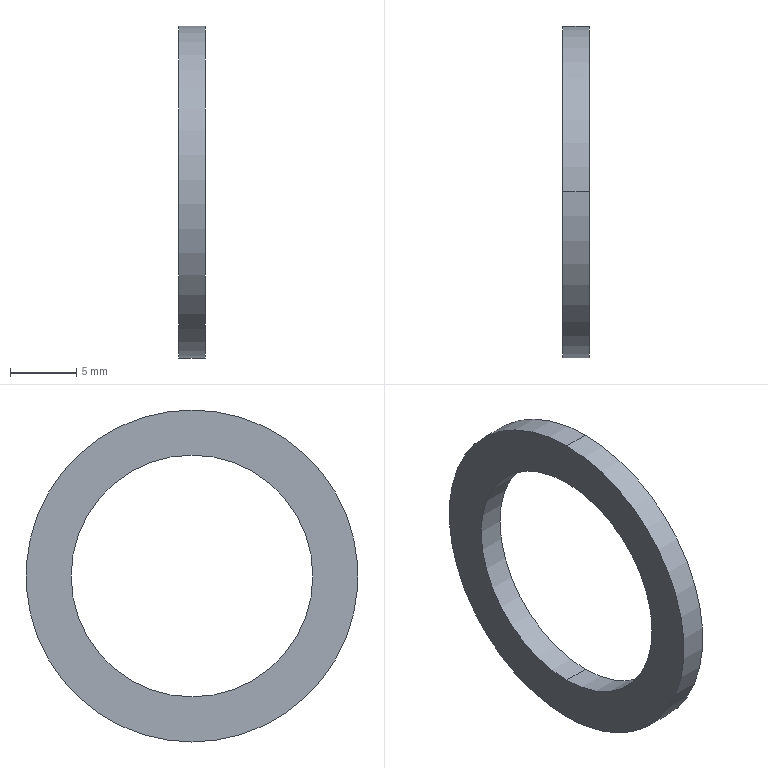Part | STEP file | PN_0010 positioning ring_Default | 1 solid | 6 faces | box 2 x 25 x 25 mm | volume 461.437 mm3 | cylinder 4 | plane 2 | commonest cylinder face diameters 18.2 x2 25 x2
STEP:
#1=CARTESIAN_POINT('',(0.,0.,0.));
#2=DIRECTION('',(0.,0.,1.));
#3=DIRECTION('',(1.,0.,0.));
#4=AXIS2_PLACEMENT_3D('',#1,#2,#3);
#5=CARTESIAN_POINT('',(2.,0.,9.1));
#6=VERTEX_POINT('',#5);
#7=CARTESIAN_POINT('',(0.,0.,9.1));
#8=VERTEX_POINT('',#7);
#9=CARTESIAN_POINT('',(2.,0.,9.1));
#10=DIRECTION('',(-1.,0.,0.));
#11=VECTOR('',#10,1.);
#12=LINE('',#9,#11);
#13=CARTESIAN_POINT('',(2.,0.,0.));
#14=DIRECTION('',(-1.,0.,0.));
#15=DIRECTION('',(0.,0.,1.));
#16=AXIS2_PLACEMENT_3D('',#13,#14,#15);
#17=CYLINDRICAL_SURFACE('',#16,9.1);
#18=CARTESIAN_POINT('',(6.283,0.));
#19=DIRECTION('',(0.,1.));
#20=VECTOR('',#19,1.);
#21=LINE('',#18,#20);
#22=(GEOMETRIC_REPRESENTATION_CONTEXT(2)PARAMETRIC_REPRESENTATION_CONTEXT()REPRESENTATION_CONTEXT('',''));
#23=DEFINITIONAL_REPRESENTATION('',(#21),#22);
#24=PCURVE('',#17,#23);
#25=CARTESIAN_POINT('',(2.,0.,0.));
#26=DIRECTION('',(-1.,0.,0.));
#27=DIRECTION('',(0.,0.,1.));
#28=AXIS2_PLACEMENT_3D('',#25,#26,#27);
#29=CYLINDRICAL_SURFACE('',#28,9.1);
#30=CARTESIAN_POINT('',(0.,0.));
#31=DIRECTION('',(0.,1.));
#32=VECTOR('',#31,1.);
#33=LINE('',#30,#32);
#34=(GEOMETRIC_REPRESENTATION_CONTEXT(2)PARAMETRIC_REPRESENTATION_CONTEXT()REPRESENTATION_CONTEXT('',''));
#35=DEFINITIONAL_REPRESENTATION('',(#33),#34);
#36=PCURVE('',#29,#35);
#37=SURFACE_CURVE('',#12,(#24,#36),.PCURVE_S1.);
#38=EDGE_CURVE('',#6,#8,#37,.T.);
#39=ORIENTED_EDGE('',*,*,#38,.T.);
#40=CARTESIAN_POINT('',(0.,0.,-9.1));
#41=VERTEX_POINT('',#40);
#42=CARTESIAN_POINT('',(0.,0.,0.));
#43=DIRECTION('',(1.,0.,0.));
#44=DIRECTION('',(0.,0.,-1.));
#45=AXIS2_PLACEMENT_3D('',#42,#43,#44);
#46=CIRCLE('',#45,9.1);
#47=CARTESIAN_POINT('',(9.425,2.));
#48=DIRECTION('',(-1.,0.));
#49=VECTOR('',#48,1.);
#50=LINE('',#47,#49);
#51=(GEOMETRIC_REPRESENTATION_CONTEXT(2)PARAMETRIC_REPRESENTATION_CONTEXT()REPRESENTATION_CONTEXT('',''));
#52=DEFINITIONAL_REPRESENTATION('',(#50),#51);
#53=PCURVE('',#17,#52);
#54=CARTESIAN_POINT('',(0.,0.,0.));
#55=DIRECTION('',(1.,0.,0.));
#56=DIRECTION('',(0.,0.,-1.));
#57=AXIS2_PLACEMENT_3D('',#54,#55,#56);
#58=PLANE('',#57);
#59=CARTESIAN_POINT('',(0.,0.));
#60=DIRECTION('',(1.,0.));
#61=AXIS2_PLACEMENT_2D('',#59,#60);
#62=CIRCLE('',#61,9.1);
#63=(GEOMETRIC_REPRESENTATION_CONTEXT(2)PARAMETRIC_REPRESENTATION_CONTEXT()REPRESENTATION_CONTEXT('',''));
#64=DEFINITIONAL_REPRESENTATION('',(#62),#63);
#65=PCURVE('',#58,#64);
#66=SURFACE_CURVE('',#46,(#53,#65),.PCURVE_S1.);
#67=EDGE_CURVE('',#8,#41,#66,.T.);
#68=ORIENTED_EDGE('',*,*,#67,.T.);
#69=CARTESIAN_POINT('',(2.,0.,-9.1));
#70=VERTEX_POINT('',#69);
#71=CARTESIAN_POINT('',(2.,0.,-9.1));
#72=DIRECTION('',(-1.,0.,0.));
#73=VECTOR('',#72,1.);
#74=LINE('',#71,#73);
#75=CARTESIAN_POINT('',(3.142,0.));
#76=DIRECTION('',(0.,1.));
#77=VECTOR('',#76,1.);
#78=LINE('',#75,#77);
#79=(GEOMETRIC_REPRESENTATION_CONTEXT(2)PARAMETRIC_REPRESENTATION_CONTEXT()REPRESENTATION_CONTEXT('',''));
#80=DEFINITIONAL_REPRESENTATION('',(#78),#79);
#81=PCURVE('',#17,#80);
#82=CARTESIAN_POINT('',(3.142,0.));
#83=DIRECTION('',(0.,1.));
#84=VECTOR('',#83,1.);
#85=LINE('',#82,#84);
#86=(GEOMETRIC_REPRESENTATION_CONTEXT(2)PARAMETRIC_REPRESENTATION_CONTEXT()REPRESENTATION_CONTEXT('',''));
#87=DEFINITIONAL_REPRESENTATION('',(#85),#86);
#88=PCURVE('',#29,#87);
#89=SURFACE_CURVE('',#74,(#81,#88),.PCURVE_S1.);
#90=EDGE_CURVE('',#70,#41,#89,.T.);
#91=ORIENTED_EDGE('',*,*,#90,.F.);
#92=CARTESIAN_POINT('',(2.,0.,0.));
#93=DIRECTION('',(1.,0.,0.));
#94=DIRECTION('',(0.,0.,-1.));
#95=AXIS2_PLACEMENT_3D('',#92,#93,#94);
#96=CIRCLE('',#95,9.1);
#97=CARTESIAN_POINT('',(9.425,0.));
#98=DIRECTION('',(-1.,0.));
#99=VECTOR('',#98,1.);
#100=LINE('',#97,#99);
#101=(GEOMETRIC_REPRESENTATION_CONTEXT(2)PARAMETRIC_REPRESENTATION_CONTEXT()REPRESENTATION_CONTEXT('',''));
#102=DEFINITIONAL_REPRESENTATION('',(#100),#101);
#103=PCURVE('',#17,#102);
#104=CARTESIAN_POINT('',(2.,0.,0.));
#105=DIRECTION('',(1.,0.,0.));
#106=DIRECTION('',(0.,0.,-1.));
#107=AXIS2_PLACEMENT_3D('',#104,#105,#106);
#108=PLANE('',#107);
#109=CARTESIAN_POINT('',(0.,0.));
#110=DIRECTION('',(1.,0.));
#111=AXIS2_PLACEMENT_2D('',#109,#110);
#112=CIRCLE('',#111,9.1);
#113=(GEOMETRIC_REPRESENTATION_CONTEXT(2)PARAMETRIC_REPRESENTATION_CONTEXT()REPRESENTATION_CONTEXT('',''));
#114=DEFINITIONAL_REPRESENTATION('',(#112),#113);
#115=PCURVE('',#108,#114);
#116=SURFACE_CURVE('',#96,(#103,#115),.PCURVE_S1.);
#117=EDGE_CURVE('',#6,#70,#116,.T.);
#118=ORIENTED_EDGE('',*,*,#117,.F.);
#119=EDGE_LOOP('',(#39,#68,#91,#118));
#120=FACE_BOUND('',#119,.F.);
#121=ADVANCED_FACE('',(#120),#17,.F.);
#122=CARTESIAN_POINT('',(2.,0.,-12.5));
#123=VERTEX_POINT('',#122);
#124=CARTESIAN_POINT('',(2.,0.,12.5));
#125=VERTEX_POINT('',#124);
#126=CARTESIAN_POINT('',(2.,0.,0.));
#127=DIRECTION('',(1.,0.,0.));
#128=DIRECTION('',(0.,0.,-1.));
#129=AXIS2_PLACEMENT_3D('',#126,#127,#128);
#130=CIRCLE('',#129,12.5);
#131=CARTESIAN_POINT('',(2.,0.,0.));
#132=DIRECTION('',(-1.,0.,0.));
#133=DIRECTION('',(0.,0.,1.));
#134=AXIS2_PLACEMENT_3D('',#131,#132,#133);
#135=CYLINDRICAL_SURFACE('',#134,12.5);
#136=CARTESIAN_POINT('',(3.142,0.));
#137=DIRECTION('',(-1.,0.));
#138=VECTOR('',#137,1.);
#139=LINE('',#136,#138);
#140=(GEOMETRIC_REPRESENTATION_CONTEXT(2)PARAMETRIC_REPRESENTATION_CONTEXT()REPRESENTATION_CONTEXT('',''));
#141=DEFINITIONAL_REPRESENTATION('',(#139),#140);
#142=PCURVE('',#135,#141);
#143=CARTESIAN_POINT('',(0.,0.));
#144=DIRECTION('',(1.,0.));
#145=AXIS2_PLACEMENT_2D('',#143,#144);
#146=CIRCLE('',#145,12.5);
#147=(GEOMETRIC_REPRESENTATION_CONTEXT(2)PARAMETRIC_REPRESENTATION_CONTEXT()REPRESENTATION_CONTEXT('',''));
#148=DEFINITIONAL_REPRESENTATION('',(#146),#147);
#149=PCURVE('',#108,#148);
#150=SURFACE_CURVE('',#130,(#142,#149),.PCURVE_S1.);
#151=EDGE_CURVE('',#123,#125,#150,.T.);
#152=ORIENTED_EDGE('',*,*,#151,.F.);
#153=CARTESIAN_POINT('',(0.,0.,-12.5));
#154=VERTEX_POINT('',#153);
#155=CARTESIAN_POINT('',(2.,0.,-12.5));
#156=DIRECTION('',(-1.,0.,0.));
#157=VECTOR('',#156,1.);
#158=LINE('',#155,#157);
#159=CARTESIAN_POINT('',(3.142,0.));
#160=DIRECTION('',(0.,1.));
#161=VECTOR('',#160,1.);
#162=LINE('',#159,#161);
#163=(GEOMETRIC_REPRESENTATION_CONTEXT(2)PARAMETRIC_REPRESENTATION_CONTEXT()REPRESENTATION_CONTEXT('',''));
#164=DEFINITIONAL_REPRESENTATION('',(#162),#163);
#165=PCURVE('',#135,#164);
#166=CARTESIAN_POINT('',(2.,0.,0.));
#167=DIRECTION('',(-1.,0.,0.));
#168=DIRECTION('',(0.,0.,1.));
#169=AXIS2_PLACEMENT_3D('',#166,#167,#168);
#170=CYLINDRICAL_SURFACE('',#169,12.5);
#171=CARTESIAN_POINT('',(3.142,0.));
#172=DIRECTION('',(0.,1.));
#173=VECTOR('',#172,1.);
#174=LINE('',#171,#173);
#175=(GEOMETRIC_REPRESENTATION_CONTEXT(2)PARAMETRIC_REPRESENTATION_CONTEXT()REPRESENTATION_CONTEXT('',''));
#176=DEFINITIONAL_REPRESENTATION('',(#174),#175);
#177=PCURVE('',#170,#176);
#178=SURFACE_CURVE('',#158,(#165,#177),.PCURVE_S1.);
#179=EDGE_CURVE('',#123,#154,#178,.T.);
#180=ORIENTED_EDGE('',*,*,#179,.T.);
#181=CARTESIAN_POINT('',(0.,0.,12.5));
#182=VERTEX_POINT('',#181);
#183=CARTESIAN_POINT('',(0.,0.,0.));
#184=DIRECTION('',(1.,0.,0.));
#185=DIRECTION('',(0.,0.,-1.));
#186=AXIS2_PLACEMENT_3D('',#183,#184,#185);
#187=CIRCLE('',#186,12.5);
#188=CARTESIAN_POINT('',(3.142,2.));
#189=DIRECTION('',(-1.,0.));
#190=VECTOR('',#189,1.);
#191=LINE('',#188,#190);
#192=(GEOMETRIC_REPRESENTATION_CONTEXT(2)PARAMETRIC_REPRESENTATION_CONTEXT()REPRESENTATION_CONTEXT('',''));
#193=DEFINITIONAL_REPRESENTATION('',(#191),#192);
#194=PCURVE('',#135,#193);
#195=CARTESIAN_POINT('',(0.,0.));
#196=DIRECTION('',(1.,0.));
#197=AXIS2_PLACEMENT_2D('',#195,#196);
#198=CIRCLE('',#197,12.5);
#199=(GEOMETRIC_REPRESENTATION_CONTEXT(2)PARAMETRIC_REPRESENTATION_CONTEXT()REPRESENTATION_CONTEXT('',''));
#200=DEFINITIONAL_REPRESENTATION('',(#198),#199);
#201=PCURVE('',#58,#200);
#202=SURFACE_CURVE('',#187,(#194,#201),.PCURVE_S1.);
#203=EDGE_CURVE('',#154,#182,#202,.T.);
#204=ORIENTED_EDGE('',*,*,#203,.T.);
#205=CARTESIAN_POINT('',(2.,0.,12.5));
#206=DIRECTION('',(-1.,0.,0.));
#207=VECTOR('',#206,1.);
#208=LINE('',#205,#207);
#209=CARTESIAN_POINT('',(0.,0.));
#210=DIRECTION('',(0.,1.));
#211=VECTOR('',#210,1.);
#212=LINE('',#209,#211);
#213=(GEOMETRIC_REPRESENTATION_CONTEXT(2)PARAMETRIC_REPRESENTATION_CONTEXT()REPRESENTATION_CONTEXT('',''));
#214=DEFINITIONAL_REPRESENTATION('',(#212),#213);
#215=PCURVE('',#135,#214);
#216=CARTESIAN_POINT('',(6.283,0.));
#217=DIRECTION('',(0.,1.));
#218=VECTOR('',#217,1.);
#219=LINE('',#216,#218);
#220=(GEOMETRIC_REPRESENTATION_CONTEXT(2)PARAMETRIC_REPRESENTATION_CONTEXT()REPRESENTATION_CONTEXT('',''));
#221=DEFINITIONAL_REPRESENTATION('',(#219),#220);
#222=PCURVE('',#170,#221);
#223=SURFACE_CURVE('',#208,(#215,#222),.PCURVE_S1.);
#224=EDGE_CURVE('',#125,#182,#223,.T.);
#225=ORIENTED_EDGE('',*,*,#224,.F.);
#226=EDGE_LOOP('',(#152,#180,#204,#225));
#227=FACE_BOUND('',#226,.T.);
#228=ADVANCED_FACE('',(#227),#135,.T.);
#229=CARTESIAN_POINT('',(2.,0.,0.));
#230=DIRECTION('',(1.,0.,0.));
#231=DIRECTION('',(0.,0.,-1.));
#232=AXIS2_PLACEMENT_3D('',#229,#230,#231);
#233=CIRCLE('',#232,12.5);
#234=CARTESIAN_POINT('',(0.,0.));
#235=DIRECTION('',(1.,0.));
#236=AXIS2_PLACEMENT_2D('',#234,#235);
#237=CIRCLE('',#236,12.5);
#238=(GEOMETRIC_REPRESENTATION_CONTEXT(2)PARAMETRIC_REPRESENTATION_CONTEXT()REPRESENTATION_CONTEXT('',''));
#239=DEFINITIONAL_REPRESENTATION('',(#237),#238);
#240=PCURVE('',#108,#239);
#241=CARTESIAN_POINT('',(9.425,0.));
#242=DIRECTION('',(-1.,0.));
#243=VECTOR('',#242,1.);
#244=LINE('',#241,#243);
#245=(GEOMETRIC_REPRESENTATION_CONTEXT(2)PARAMETRIC_REPRESENTATION_CONTEXT()REPRESENTATION_CONTEXT('',''));
#246=DEFINITIONAL_REPRESENTATION('',(#244),#245);
#247=PCURVE('',#170,#246);
#248=SURFACE_CURVE('',#233,(#240,#247),.PCURVE_S1.);
#249=EDGE_CURVE('',#125,#123,#248,.T.);
#250=ORIENTED_EDGE('',*,*,#249,.T.);
#251=ORIENTED_EDGE('',*,*,#151,.T.);
#252=EDGE_LOOP('',(#250,#251));
#253=FACE_BOUND('',#252,.T.);
#254=ORIENTED_EDGE('',*,*,#117,.F.);
#255=CARTESIAN_POINT('',(2.,0.,0.));
#256=DIRECTION('',(1.,0.,0.));
#257=DIRECTION('',(0.,0.,-1.));
#258=AXIS2_PLACEMENT_3D('',#255,#256,#257);
#259=CIRCLE('',#258,9.1);
#260=CARTESIAN_POINT('',(0.,0.));
#261=DIRECTION('',(1.,0.));
#262=AXIS2_PLACEMENT_2D('',#260,#261);
#263=CIRCLE('',#262,9.1);
#264=(GEOMETRIC_REPRESENTATION_CONTEXT(2)PARAMETRIC_REPRESENTATION_CONTEXT()REPRESENTATION_CONTEXT('',''));
#265=DEFINITIONAL_REPRESENTATION('',(#263),#264);
#266=PCURVE('',#108,#265);
#267=CARTESIAN_POINT('',(3.142,0.));
#268=DIRECTION('',(-1.,0.));
#269=VECTOR('',#268,1.);
#270=LINE('',#267,#269);
#271=(GEOMETRIC_REPRESENTATION_CONTEXT(2)PARAMETRIC_REPRESENTATION_CONTEXT()REPRESENTATION_CONTEXT('',''));
#272=DEFINITIONAL_REPRESENTATION('',(#270),#271);
#273=PCURVE('',#29,#272);
#274=SURFACE_CURVE('',#259,(#266,#273),.PCURVE_S1.);
#275=EDGE_CURVE('',#70,#6,#274,.T.);
#276=ORIENTED_EDGE('',*,*,#275,.F.);
#277=EDGE_LOOP('',(#254,#276));
#278=FACE_BOUND('',#277,.T.);
#279=ADVANCED_FACE('',(#253,#278),#108,.T.);
#280=CARTESIAN_POINT('',(0.,0.,0.));
#281=DIRECTION('',(1.,0.,0.));
#282=DIRECTION('',(0.,0.,-1.));
#283=AXIS2_PLACEMENT_3D('',#280,#281,#282);
#284=CIRCLE('',#283,12.5);
#285=CARTESIAN_POINT('',(0.,0.));
#286=DIRECTION('',(1.,0.));
#287=AXIS2_PLACEMENT_2D('',#285,#286);
#288=CIRCLE('',#287,12.5);
#289=(GEOMETRIC_REPRESENTATION_CONTEXT(2)PARAMETRIC_REPRESENTATION_CONTEXT()REPRESENTATION_CONTEXT('',''));
#290=DEFINITIONAL_REPRESENTATION('',(#288),#289);
#291=PCURVE('',#58,#290);
#292=CARTESIAN_POINT('',(9.425,2.));
#293=DIRECTION('',(-1.,0.));
#294=VECTOR('',#293,1.);
#295=LINE('',#292,#294);
#296=(GEOMETRIC_REPRESENTATION_CONTEXT(2)PARAMETRIC_REPRESENTATION_CONTEXT()REPRESENTATION_CONTEXT('',''));
#297=DEFINITIONAL_REPRESENTATION('',(#295),#296);
#298=PCURVE('',#170,#297);
#299=SURFACE_CURVE('',#284,(#291,#298),.PCURVE_S1.);
#300=EDGE_CURVE('',#182,#154,#299,.T.);
#301=ORIENTED_EDGE('',*,*,#300,.F.);
#302=ORIENTED_EDGE('',*,*,#203,.F.);
#303=EDGE_LOOP('',(#301,#302));
#304=FACE_BOUND('',#303,.T.);
#305=ORIENTED_EDGE('',*,*,#67,.T.);
#306=CARTESIAN_POINT('',(0.,0.,0.));
#307=DIRECTION('',(1.,0.,0.));
#308=DIRECTION('',(0.,0.,-1.));
#309=AXIS2_PLACEMENT_3D('',#306,#307,#308);
#310=CIRCLE('',#309,9.1);
#311=CARTESIAN_POINT('',(0.,0.));
#312=DIRECTION('',(1.,0.));
#313=AXIS2_PLACEMENT_2D('',#311,#312);
#314=CIRCLE('',#313,9.1);
#315=(GEOMETRIC_REPRESENTATION_CONTEXT(2)PARAMETRIC_REPRESENTATION_CONTEXT()REPRESENTATION_CONTEXT('',''));
#316=DEFINITIONAL_REPRESENTATION('',(#314),#315);
#317=PCURVE('',#58,#316);
#318=CARTESIAN_POINT('',(3.142,2.));
#319=DIRECTION('',(-1.,0.));
#320=VECTOR('',#319,1.);
#321=LINE('',#318,#320);
#322=(GEOMETRIC_REPRESENTATION_CONTEXT(2)PARAMETRIC_REPRESENTATION_CONTEXT()REPRESENTATION_CONTEXT('',''));
#323=DEFINITIONAL_REPRESENTATION('',(#321),#322);
#324=PCURVE('',#29,#323);
#325=SURFACE_CURVE('',#310,(#317,#324),.PCURVE_S1.);
#326=EDGE_CURVE('',#41,#8,#325,.T.);
#327=ORIENTED_EDGE('',*,*,#326,.T.);
#328=EDGE_LOOP('',(#305,#327));
#329=FACE_BOUND('',#328,.T.);
#330=ADVANCED_FACE('',(#304,#329),#58,.F.);
#331=ORIENTED_EDGE('',*,*,#179,.F.);
#332=ORIENTED_EDGE('',*,*,#249,.F.);
#333=ORIENTED_EDGE('',*,*,#224,.T.);
#334=ORIENTED_EDGE('',*,*,#300,.T.);
#335=EDGE_LOOP('',(#331,#332,#333,#334));
#336=FACE_BOUND('',#335,.T.);
#337=ADVANCED_FACE('',(#336),#170,.T.);
#338=ORIENTED_EDGE('',*,*,#326,.T.);
#339=ORIENTED_EDGE('',*,*,#38,.F.);
#340=ORIENTED_EDGE('',*,*,#275,.F.);
#341=ORIENTED_EDGE('',*,*,#90,.T.);
#342=EDGE_LOOP('',(#338,#339,#340,#341));
#343=FACE_BOUND('',#342,.F.);
#344=ADVANCED_FACE('',(#343),#29,.F.);
#345=CLOSED_SHELL('',(#121,#228,#279,#330,#337,#344));
#346=MANIFOLD_SOLID_BREP('',#345);
#347=(LENGTH_UNIT()NAMED_UNIT(*)SI_UNIT(.MILLI.,.METRE.));
#348=UNCERTAINTY_MEASURE_WITH_UNIT(LENGTH_MEASURE(0.0000001),#347,'','');
#349=(NAMED_UNIT(*)PLANE_ANGLE_UNIT()SI_UNIT($,.RADIAN.));
#350=(NAMED_UNIT(*)SI_UNIT($,.STERADIAN.)SOLID_ANGLE_UNIT());
#351=(GEOMETRIC_REPRESENTATION_CONTEXT(3)GLOBAL_UNCERTAINTY_ASSIGNED_CONTEXT((#348))GLOBAL_UNIT_ASSIGNED_CONTEXT((#347,#349,#350))REPRESENTATION_CONTEXT('',''));
#352=ADVANCED_BREP_SHAPE_REPRESENTATION('',(#4,#346),#351);